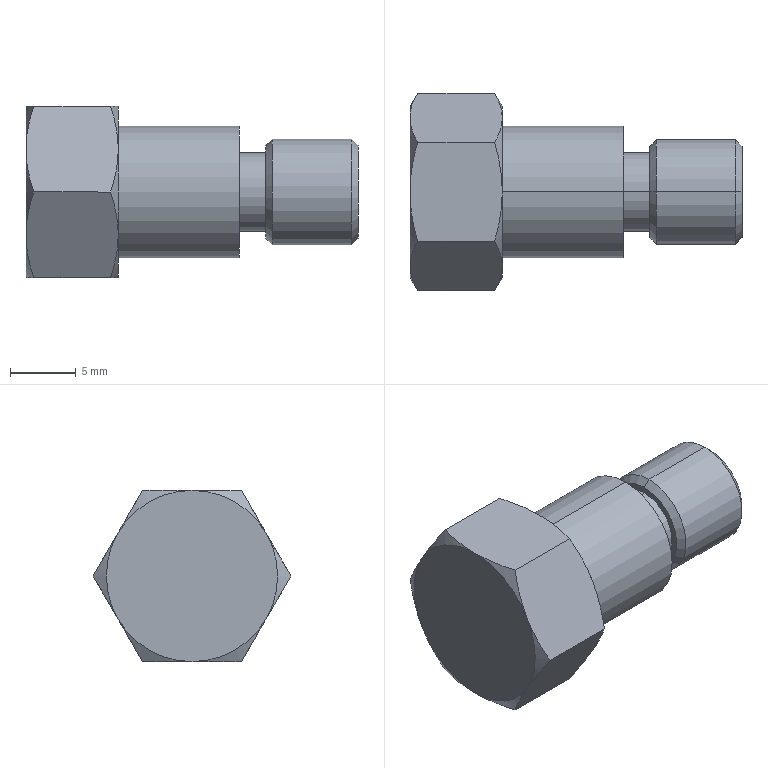Part | STEP file | Tray bolt | 1 solid | 33 faces | box 25.2 x 15.011 x 13 mm | volume 2145 mm3 | cone 16 | plane 11 | cylinder 6 | commonest cylinder face diameters 6 x2 8 x2 10 x2